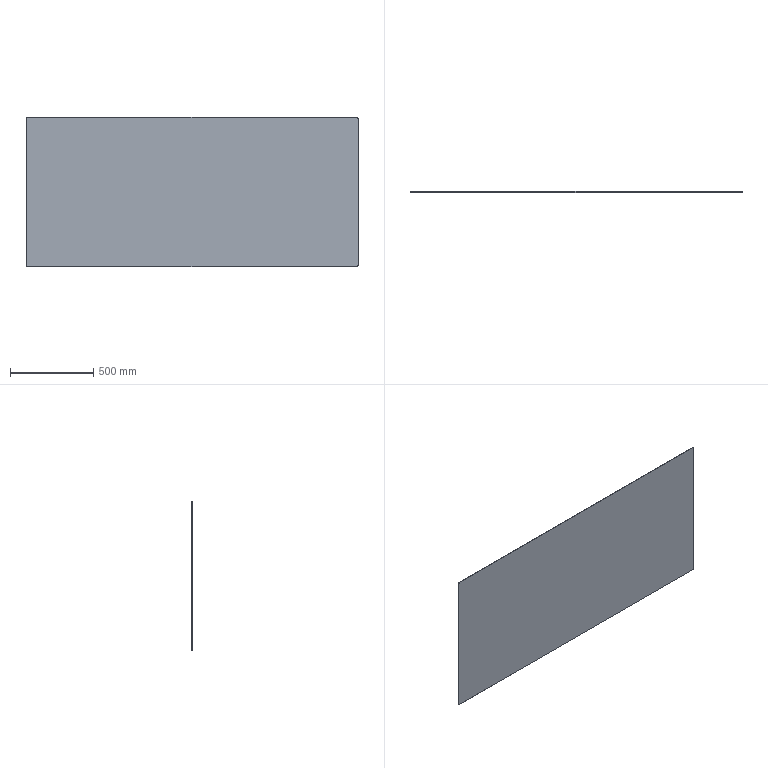Part | SolidWorks | features Extrusion 1, Fillet 1 | 1 solid | 10 faces | box 2000 x 5 x 900 mm | volume 8999845 mm3 | plane 6 | cylinder 4 | commonest cylinder face diameters 12 x4
STEP:
#1=CARTESIAN_POINT('',(1000.,5.,444.));
#2=VERTEX_POINT('',#1);
#3=CARTESIAN_POINT('',(1000.,5.,-444.));
#4=VERTEX_POINT('',#3);
#5=CARTESIAN_POINT('',(1000.,5.,-450.));
#6=DIRECTION('',(0.,0.,-1.));
#7=VECTOR('',#6,1000.);
#8=LINE('',#5,#7);
#9=EDGE_CURVE('',#2,#4,#8,.T.);
#10=ORIENTED_EDGE('',*,*,#9,.F.);
#11=CARTESIAN_POINT('',(1000.,0.,444.));
#12=VERTEX_POINT('',#11);
#13=CARTESIAN_POINT('',(1000.,5.,444.));
#14=DIRECTION('',(0.,-1.,0.));
#15=VECTOR('',#14,1000.);
#16=LINE('',#13,#15);
#17=EDGE_CURVE('',#2,#12,#16,.T.);
#18=ORIENTED_EDGE('',*,*,#17,.T.);
#19=CARTESIAN_POINT('',(1000.,0.,-444.));
#20=VERTEX_POINT('',#19);
#21=CARTESIAN_POINT('',(1000.,0.,-450.));
#22=DIRECTION('',(0.,0.,-1.));
#23=VECTOR('',#22,1000.);
#24=LINE('',#21,#23);
#25=EDGE_CURVE('',#12,#20,#24,.T.);
#26=ORIENTED_EDGE('',*,*,#25,.T.);
#27=CARTESIAN_POINT('',(1000.,5.,-444.));
#28=DIRECTION('',(0.,1.,0.));
#29=VECTOR('',#28,1000.);
#30=LINE('',#27,#29);
#31=EDGE_CURVE('',#20,#4,#30,.T.);
#32=ORIENTED_EDGE('',*,*,#31,.T.);
#33=EDGE_LOOP('',(#10,#18,#26,#32));
#34=FACE_OUTER_BOUND('',#33,.T.);
#35=CARTESIAN_POINT('',(1000.,5.,-450.));
#36=DIRECTION('',(-1.,0.,0.));
#37=DIRECTION('',(0.,0.,1.));
#38=AXIS2_PLACEMENT_3D('',#35,#36,#37);
#39=PLANE('',#38);
#40=ADVANCED_FACE('',(#34),#39,.F.);
#41=CARTESIAN_POINT('',(994.,5.,-450.));
#42=VERTEX_POINT('',#41);
#43=CARTESIAN_POINT('',(-994.,5.,-450.));
#44=VERTEX_POINT('',#43);
#45=CARTESIAN_POINT('',(-1000.,5.,-450.));
#46=DIRECTION('',(-1.,0.,0.));
#47=VECTOR('',#46,1000.);
#48=LINE('',#45,#47);
#49=EDGE_CURVE('',#42,#44,#48,.T.);
#50=ORIENTED_EDGE('',*,*,#49,.F.);
#51=CARTESIAN_POINT('',(994.,0.,-450.));
#52=VERTEX_POINT('',#51);
#53=CARTESIAN_POINT('',(994.,5.,-450.));
#54=DIRECTION('',(0.,-1.,0.));
#55=VECTOR('',#54,1000.);
#56=LINE('',#53,#55);
#57=EDGE_CURVE('',#42,#52,#56,.T.);
#58=ORIENTED_EDGE('',*,*,#57,.T.);
#59=CARTESIAN_POINT('',(-994.,0.,-450.));
#60=VERTEX_POINT('',#59);
#61=CARTESIAN_POINT('',(-1000.,0.,-450.));
#62=DIRECTION('',(-1.,0.,0.));
#63=VECTOR('',#62,1000.);
#64=LINE('',#61,#63);
#65=EDGE_CURVE('',#52,#60,#64,.T.);
#66=ORIENTED_EDGE('',*,*,#65,.T.);
#67=CARTESIAN_POINT('',(-994.,5.,-450.));
#68=DIRECTION('',(0.,1.,0.));
#69=VECTOR('',#68,1000.);
#70=LINE('',#67,#69);
#71=EDGE_CURVE('',#60,#44,#70,.T.);
#72=ORIENTED_EDGE('',*,*,#71,.T.);
#73=EDGE_LOOP('',(#50,#58,#66,#72));
#74=FACE_OUTER_BOUND('',#73,.T.);
#75=CARTESIAN_POINT('',(-1000.,5.,-450.));
#76=DIRECTION('',(0.,0.,1.));
#77=DIRECTION('',(1.,0.,0.));
#78=AXIS2_PLACEMENT_3D('',#75,#76,#77);
#79=PLANE('',#78);
#80=ADVANCED_FACE('',(#74),#79,.F.);
#81=CARTESIAN_POINT('',(-1000.,0.,-444.));
#82=VERTEX_POINT('',#81);
#83=CARTESIAN_POINT('',(-1000.,0.,444.));
#84=VERTEX_POINT('',#83);
#85=CARTESIAN_POINT('',(-1000.,0.,-450.));
#86=DIRECTION('',(0.,0.,1.));
#87=VECTOR('',#86,1000.);
#88=LINE('',#85,#87);
#89=EDGE_CURVE('',#82,#84,#88,.T.);
#90=ORIENTED_EDGE('',*,*,#89,.T.);
#91=CARTESIAN_POINT('',(-1000.,5.,444.));
#92=VERTEX_POINT('',#91);
#93=CARTESIAN_POINT('',(-1000.,5.,444.));
#94=DIRECTION('',(0.,1.,0.));
#95=VECTOR('',#94,1000.);
#96=LINE('',#93,#95);
#97=EDGE_CURVE('',#84,#92,#96,.T.);
#98=ORIENTED_EDGE('',*,*,#97,.T.);
#99=CARTESIAN_POINT('',(-1000.,5.,-444.));
#100=VERTEX_POINT('',#99);
#101=CARTESIAN_POINT('',(-1000.,5.,-450.));
#102=DIRECTION('',(0.,0.,1.));
#103=VECTOR('',#102,1000.);
#104=LINE('',#101,#103);
#105=EDGE_CURVE('',#100,#92,#104,.T.);
#106=ORIENTED_EDGE('',*,*,#105,.F.);
#107=CARTESIAN_POINT('',(-1000.,5.,-444.));
#108=DIRECTION('',(0.,-1.,0.));
#109=VECTOR('',#108,1000.);
#110=LINE('',#107,#109);
#111=EDGE_CURVE('',#100,#82,#110,.T.);
#112=ORIENTED_EDGE('',*,*,#111,.T.);
#113=EDGE_LOOP('',(#90,#98,#106,#112));
#114=FACE_OUTER_BOUND('',#113,.T.);
#115=CARTESIAN_POINT('',(-1000.,5.,-450.));
#116=DIRECTION('',(1.,0.,0.));
#117=DIRECTION('',(0.,0.,-1.));
#118=AXIS2_PLACEMENT_3D('',#115,#116,#117);
#119=PLANE('',#118);
#120=ADVANCED_FACE('',(#114),#119,.F.);
#121=CARTESIAN_POINT('',(-994.,5.,450.));
#122=VERTEX_POINT('',#121);
#123=CARTESIAN_POINT('',(994.,5.,450.));
#124=VERTEX_POINT('',#123);
#125=CARTESIAN_POINT('',(-1000.,5.,450.));
#126=DIRECTION('',(1.,0.,0.));
#127=VECTOR('',#126,1000.);
#128=LINE('',#125,#127);
#129=EDGE_CURVE('',#122,#124,#128,.T.);
#130=ORIENTED_EDGE('',*,*,#129,.F.);
#131=CARTESIAN_POINT('',(-994.,0.,450.));
#132=VERTEX_POINT('',#131);
#133=CARTESIAN_POINT('',(-994.,5.,450.));
#134=DIRECTION('',(0.,-1.,0.));
#135=VECTOR('',#134,1000.);
#136=LINE('',#133,#135);
#137=EDGE_CURVE('',#122,#132,#136,.T.);
#138=ORIENTED_EDGE('',*,*,#137,.T.);
#139=CARTESIAN_POINT('',(994.,0.,450.));
#140=VERTEX_POINT('',#139);
#141=CARTESIAN_POINT('',(-1000.,0.,450.));
#142=DIRECTION('',(1.,0.,0.));
#143=VECTOR('',#142,1000.);
#144=LINE('',#141,#143);
#145=EDGE_CURVE('',#132,#140,#144,.T.);
#146=ORIENTED_EDGE('',*,*,#145,.T.);
#147=CARTESIAN_POINT('',(994.,5.,450.));
#148=DIRECTION('',(0.,1.,0.));
#149=VECTOR('',#148,1000.);
#150=LINE('',#147,#149);
#151=EDGE_CURVE('',#140,#124,#150,.T.);
#152=ORIENTED_EDGE('',*,*,#151,.T.);
#153=EDGE_LOOP('',(#130,#138,#146,#152));
#154=FACE_OUTER_BOUND('',#153,.T.);
#155=CARTESIAN_POINT('',(-1000.,5.,450.));
#156=DIRECTION('',(0.,0.,-1.));
#157=DIRECTION('',(-1.,0.,0.));
#158=AXIS2_PLACEMENT_3D('',#155,#156,#157);
#159=PLANE('',#158);
#160=ADVANCED_FACE('',(#154),#159,.F.);
#161=ORIENTED_EDGE('',*,*,#105,.T.);
#162=CARTESIAN_POINT('',(-994.,5.,444.));
#163=DIRECTION('',(0.,1.,0.));
#164=DIRECTION('',(0.,0.,1.));
#165=AXIS2_PLACEMENT_3D('',#162,#163,#164);
#166=CIRCLE('',#165,6.);
#167=EDGE_CURVE('',#92,#122,#166,.T.);
#168=ORIENTED_EDGE('',*,*,#167,.T.);
#169=ORIENTED_EDGE('',*,*,#129,.T.);
#170=CARTESIAN_POINT('',(994.,5.,444.));
#171=DIRECTION('',(0.,1.,0.));
#172=DIRECTION('',(0.,0.,1.));
#173=AXIS2_PLACEMENT_3D('',#170,#171,#172);
#174=CIRCLE('',#173,6.);
#175=EDGE_CURVE('',#124,#2,#174,.T.);
#176=ORIENTED_EDGE('',*,*,#175,.T.);
#177=ORIENTED_EDGE('',*,*,#9,.T.);
#178=CARTESIAN_POINT('',(994.,5.,-444.));
#179=DIRECTION('',(0.,1.,0.));
#180=DIRECTION('',(0.,0.,1.));
#181=AXIS2_PLACEMENT_3D('',#178,#179,#180);
#182=CIRCLE('',#181,6.);
#183=EDGE_CURVE('',#4,#42,#182,.T.);
#184=ORIENTED_EDGE('',*,*,#183,.T.);
#185=ORIENTED_EDGE('',*,*,#49,.T.);
#186=CARTESIAN_POINT('',(-994.,5.,-444.));
#187=DIRECTION('',(0.,1.,0.));
#188=DIRECTION('',(0.,0.,1.));
#189=AXIS2_PLACEMENT_3D('',#186,#187,#188);
#190=CIRCLE('',#189,6.);
#191=EDGE_CURVE('',#44,#100,#190,.T.);
#192=ORIENTED_EDGE('',*,*,#191,.T.);
#193=EDGE_LOOP('',(#161,#168,#169,#176,#177,#184,#185,#192));
#194=FACE_OUTER_BOUND('',#193,.T.);
#195=CARTESIAN_POINT('',(0.,5.,0.));
#196=DIRECTION('',(0.,1.,0.));
#197=DIRECTION('',(0.,0.,1.));
#198=AXIS2_PLACEMENT_3D('',#195,#196,#197);
#199=PLANE('',#198);
#200=ADVANCED_FACE('',(#194),#199,.T.);
#201=ORIENTED_EDGE('',*,*,#145,.F.);
#202=CARTESIAN_POINT('',(-994.,0.,444.));
#203=DIRECTION('',(0.,-1.,0.));
#204=DIRECTION('',(0.,0.,1.));
#205=AXIS2_PLACEMENT_3D('',#202,#203,#204);
#206=CIRCLE('',#205,6.);
#207=EDGE_CURVE('',#132,#84,#206,.T.);
#208=ORIENTED_EDGE('',*,*,#207,.T.);
#209=ORIENTED_EDGE('',*,*,#89,.F.);
#210=CARTESIAN_POINT('',(-994.,0.,-444.));
#211=DIRECTION('',(0.,-1.,0.));
#212=DIRECTION('',(0.,0.,1.));
#213=AXIS2_PLACEMENT_3D('',#210,#211,#212);
#214=CIRCLE('',#213,6.);
#215=EDGE_CURVE('',#82,#60,#214,.T.);
#216=ORIENTED_EDGE('',*,*,#215,.T.);
#217=ORIENTED_EDGE('',*,*,#65,.F.);
#218=CARTESIAN_POINT('',(994.,0.,-444.));
#219=DIRECTION('',(0.,-1.,0.));
#220=DIRECTION('',(0.,0.,1.));
#221=AXIS2_PLACEMENT_3D('',#218,#219,#220);
#222=CIRCLE('',#221,6.);
#223=EDGE_CURVE('',#52,#20,#222,.T.);
#224=ORIENTED_EDGE('',*,*,#223,.T.);
#225=ORIENTED_EDGE('',*,*,#25,.F.);
#226=CARTESIAN_POINT('',(994.,0.,444.));
#227=DIRECTION('',(0.,-1.,0.));
#228=DIRECTION('',(0.,0.,1.));
#229=AXIS2_PLACEMENT_3D('',#226,#227,#228);
#230=CIRCLE('',#229,6.);
#231=EDGE_CURVE('',#12,#140,#230,.T.);
#232=ORIENTED_EDGE('',*,*,#231,.T.);
#233=EDGE_LOOP('',(#201,#208,#209,#216,#217,#224,#225,#232));
#234=FACE_OUTER_BOUND('',#233,.T.);
#235=CARTESIAN_POINT('',(0.,0.,0.));
#236=DIRECTION('',(0.,1.,0.));
#237=DIRECTION('',(0.,0.,1.));
#238=AXIS2_PLACEMENT_3D('',#235,#236,#237);
#239=PLANE('',#238);
#240=ADVANCED_FACE('',(#234),#239,.F.);
#241=ORIENTED_EDGE('',*,*,#167,.F.);
#242=ORIENTED_EDGE('',*,*,#97,.F.);
#243=ORIENTED_EDGE('',*,*,#207,.F.);
#244=ORIENTED_EDGE('',*,*,#137,.F.);
#245=EDGE_LOOP('',(#241,#242,#243,#244));
#246=FACE_OUTER_BOUND('',#245,.T.);
#247=CARTESIAN_POINT('',(-994.,5.,444.));
#248=DIRECTION('',(0.,-1.,0.));
#249=DIRECTION('',(0.,0.,-1.));
#250=AXIS2_PLACEMENT_3D('',#247,#248,#249);
#251=CYLINDRICAL_SURFACE('',#250,6.);
#252=ADVANCED_FACE('',(#246),#251,.T.);
#253=ORIENTED_EDGE('',*,*,#175,.F.);
#254=ORIENTED_EDGE('',*,*,#151,.F.);
#255=ORIENTED_EDGE('',*,*,#231,.F.);
#256=ORIENTED_EDGE('',*,*,#17,.F.);
#257=EDGE_LOOP('',(#253,#254,#255,#256));
#258=FACE_OUTER_BOUND('',#257,.T.);
#259=CARTESIAN_POINT('',(994.,5.,444.));
#260=DIRECTION('',(0.,-1.,0.));
#261=DIRECTION('',(0.,0.,-1.));
#262=AXIS2_PLACEMENT_3D('',#259,#260,#261);
#263=CYLINDRICAL_SURFACE('',#262,6.);
#264=ADVANCED_FACE('',(#258),#263,.T.);
#265=ORIENTED_EDGE('',*,*,#183,.F.);
#266=ORIENTED_EDGE('',*,*,#31,.F.);
#267=ORIENTED_EDGE('',*,*,#223,.F.);
#268=ORIENTED_EDGE('',*,*,#57,.F.);
#269=EDGE_LOOP('',(#265,#266,#267,#268));
#270=FACE_OUTER_BOUND('',#269,.T.);
#271=CARTESIAN_POINT('',(994.,5.,-444.));
#272=DIRECTION('',(0.,-1.,0.));
#273=DIRECTION('',(0.,0.,-1.));
#274=AXIS2_PLACEMENT_3D('',#271,#272,#273);
#275=CYLINDRICAL_SURFACE('',#274,6.);
#276=ADVANCED_FACE('',(#270),#275,.T.);
#277=ORIENTED_EDGE('',*,*,#191,.F.);
#278=ORIENTED_EDGE('',*,*,#71,.F.);
#279=ORIENTED_EDGE('',*,*,#215,.F.);
#280=ORIENTED_EDGE('',*,*,#111,.F.);
#281=EDGE_LOOP('',(#277,#278,#279,#280));
#282=FACE_OUTER_BOUND('',#281,.T.);
#283=CARTESIAN_POINT('',(-994.,5.,-444.));
#284=DIRECTION('',(0.,-1.,0.));
#285=DIRECTION('',(0.,0.,-1.));
#286=AXIS2_PLACEMENT_3D('',#283,#284,#285);
#287=CYLINDRICAL_SURFACE('',#286,6.);
#288=ADVANCED_FACE('',(#282),#287,.T.);
#289=CLOSED_SHELL('',(#40,#80,#120,#160,#200,#240,#252,#264,#276,#288));
#290=MANIFOLD_SOLID_BREP('',#289);
#291=CARTESIAN_POINT('',(0.,0.,0.));
#292=DIRECTION('',(0.,0.,1.));
#293=DIRECTION('',(1.,0.,0.));
#294=AXIS2_PLACEMENT_3D('',#291,#292,#293);
#295=(LENGTH_UNIT()NAMED_UNIT(*)SI_UNIT(.MILLI.,.METRE.));
#296=UNCERTAINTY_MEASURE_WITH_UNIT(LENGTH_MEASURE(0.00001),#295,'','');
#297=(NAMED_UNIT(*)PLANE_ANGLE_UNIT()SI_UNIT($,.RADIAN.));
#298=(NAMED_UNIT(*)SI_UNIT($,.STERADIAN.)SOLID_ANGLE_UNIT());
#299=(GEOMETRIC_REPRESENTATION_CONTEXT(3)GLOBAL_UNCERTAINTY_ASSIGNED_CONTEXT((#296))GLOBAL_UNIT_ASSIGNED_CONTEXT((#295,#297,#298))REPRESENTATION_CONTEXT('',''));
#300=ADVANCED_BREP_SHAPE_REPRESENTATION('',(#290,#294),#299);